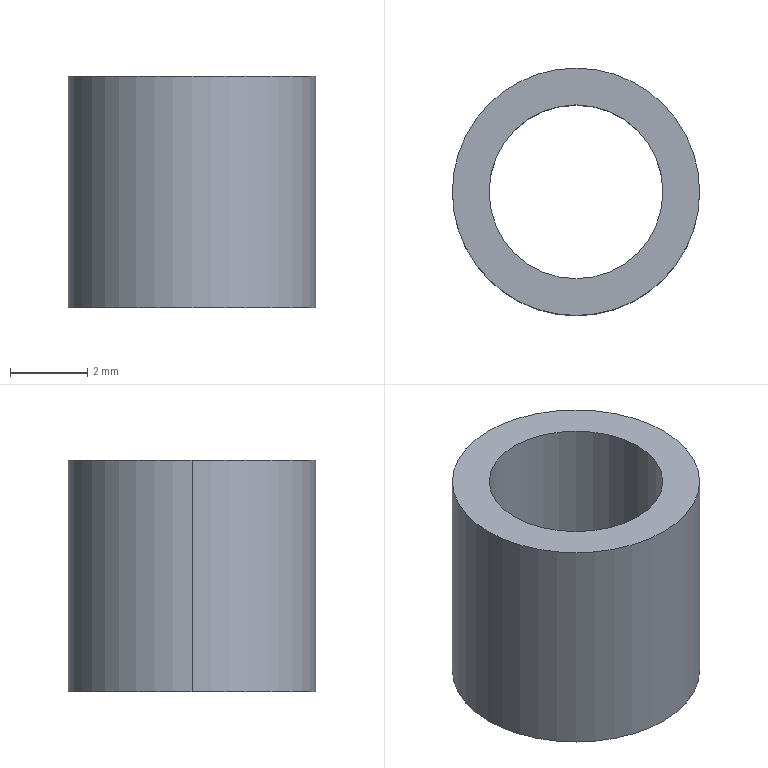Part | NX | features BREP 1 | 1 solid | 6 faces | box 6.4 x 6.4 x 6 mm | volume 97.594 mm3 | cylinder 4 | plane 2 | commonest cylinder face diameters 4.5 x2 6.4 x2
STEP:
#1=CARTESIAN_POINT('',(11.941,-8.741,33.83));
#2=VERTEX_POINT('',#1);
#3=CARTESIAN_POINT('',(5.541,-8.741,33.83));
#4=VERTEX_POINT('',#3);
#5=CARTESIAN_POINT('',(8.741,-8.741,33.83));
#6=DIRECTION('',(0.,0.,1.));
#7=DIRECTION('',(1.,0.,0.));
#8=AXIS2_PLACEMENT_3D('',#5,#6,#7);
#9=CIRCLE('',#8,3.2);
#10=EDGE_CURVE('',#2,#4,#9,.T.);
#11=ORIENTED_EDGE('',*,*,#10,.T.);
#12=CARTESIAN_POINT('',(8.741,-8.741,33.83));
#13=DIRECTION('',(0.,0.,1.));
#14=DIRECTION('',(-1.,0.,0.));
#15=AXIS2_PLACEMENT_3D('',#12,#13,#14);
#16=CIRCLE('',#15,3.2);
#17=EDGE_CURVE('',#4,#2,#16,.T.);
#18=ORIENTED_EDGE('',*,*,#17,.T.);
#19=EDGE_LOOP('',(#11,#18));
#20=FACE_BOUND('',#19,.T.);
#21=CARTESIAN_POINT('',(10.991,-8.741,33.83));
#22=VERTEX_POINT('',#21);
#23=CARTESIAN_POINT('',(6.491,-8.741,33.83));
#24=VERTEX_POINT('',#23);
#25=CARTESIAN_POINT('',(8.741,-8.741,33.83));
#26=DIRECTION('',(0.,0.,-1.));
#27=DIRECTION('',(1.,0.,0.));
#28=AXIS2_PLACEMENT_3D('',#25,#26,#27);
#29=CIRCLE('',#28,2.25);
#30=EDGE_CURVE('',#22,#24,#29,.T.);
#31=ORIENTED_EDGE('',*,*,#30,.T.);
#32=CARTESIAN_POINT('',(8.741,-8.741,33.83));
#33=DIRECTION('',(0.,0.,-1.));
#34=DIRECTION('',(-1.,0.,0.));
#35=AXIS2_PLACEMENT_3D('',#32,#33,#34);
#36=CIRCLE('',#35,2.25);
#37=EDGE_CURVE('',#24,#22,#36,.T.);
#38=ORIENTED_EDGE('',*,*,#37,.T.);
#39=EDGE_LOOP('',(#31,#38));
#40=FACE_BOUND('',#39,.T.);
#41=CARTESIAN_POINT('',(0.,0.,33.83));
#42=DIRECTION('',(0.,0.,1.));
#43=DIRECTION('',(1.,0.,0.));
#44=AXIS2_PLACEMENT_3D('',#41,#42,#43);
#45=PLANE('',#44);
#46=ADVANCED_FACE('',(#20,#40),#45,.T.);
#47=CARTESIAN_POINT('',(11.941,-8.741,27.83));
#48=VERTEX_POINT('',#47);
#49=CARTESIAN_POINT('',(5.541,-8.741,27.83));
#50=VERTEX_POINT('',#49);
#51=CARTESIAN_POINT('',(8.741,-8.741,27.83));
#52=DIRECTION('',(0.,0.,-1.));
#53=DIRECTION('',(1.,0.,0.));
#54=AXIS2_PLACEMENT_3D('',#51,#52,#53);
#55=CIRCLE('',#54,3.2);
#56=EDGE_CURVE('',#48,#50,#55,.T.);
#57=ORIENTED_EDGE('',*,*,#56,.F.);
#58=CARTESIAN_POINT('',(11.941,-8.741,33.83));
#59=DIRECTION('',(0.,0.,-1.));
#60=VECTOR('',#59,1000.);
#61=LINE('',#58,#60);
#62=EDGE_CURVE('',#2,#48,#61,.T.);
#63=ORIENTED_EDGE('',*,*,#62,.F.);
#64=ORIENTED_EDGE('',*,*,#17,.F.);
#65=CARTESIAN_POINT('',(5.541,-8.741,33.83));
#66=DIRECTION('',(0.,0.,-1.));
#67=VECTOR('',#66,1000.);
#68=LINE('',#65,#67);
#69=EDGE_CURVE('',#4,#50,#68,.T.);
#70=ORIENTED_EDGE('',*,*,#69,.T.);
#71=EDGE_LOOP('',(#57,#63,#64,#70));
#72=FACE_BOUND('',#71,.T.);
#73=CARTESIAN_POINT('',(8.741,-8.741,33.83));
#74=DIRECTION('',(0.,0.,1.));
#75=DIRECTION('',(1.,0.,0.));
#76=AXIS2_PLACEMENT_3D('',#73,#74,#75);
#77=CYLINDRICAL_SURFACE('',#76,3.2);
#78=ADVANCED_FACE('',(#72),#77,.T.);
#79=CARTESIAN_POINT('',(8.741,-8.741,27.83));
#80=DIRECTION('',(0.,0.,-1.));
#81=DIRECTION('',(-1.,0.,0.));
#82=AXIS2_PLACEMENT_3D('',#79,#80,#81);
#83=CIRCLE('',#82,3.2);
#84=EDGE_CURVE('',#50,#48,#83,.T.);
#85=ORIENTED_EDGE('',*,*,#84,.F.);
#86=ORIENTED_EDGE('',*,*,#69,.F.);
#87=ORIENTED_EDGE('',*,*,#10,.F.);
#88=ORIENTED_EDGE('',*,*,#62,.T.);
#89=EDGE_LOOP('',(#85,#86,#87,#88));
#90=FACE_BOUND('',#89,.T.);
#91=CARTESIAN_POINT('',(8.741,-8.741,33.83));
#92=DIRECTION('',(0.,0.,1.));
#93=DIRECTION('',(1.,0.,0.));
#94=AXIS2_PLACEMENT_3D('',#91,#92,#93);
#95=CYLINDRICAL_SURFACE('',#94,3.2);
#96=ADVANCED_FACE('',(#90),#95,.T.);
#97=ORIENTED_EDGE('',*,*,#84,.T.);
#98=ORIENTED_EDGE('',*,*,#56,.T.);
#99=EDGE_LOOP('',(#97,#98));
#100=FACE_BOUND('',#99,.T.);
#101=CARTESIAN_POINT('',(6.491,-8.741,27.83));
#102=VERTEX_POINT('',#101);
#103=CARTESIAN_POINT('',(10.991,-8.741,27.83));
#104=VERTEX_POINT('',#103);
#105=CARTESIAN_POINT('',(8.741,-8.741,27.83));
#106=DIRECTION('',(0.,0.,1.));
#107=DIRECTION('',(-1.,0.,0.));
#108=AXIS2_PLACEMENT_3D('',#105,#106,#107);
#109=CIRCLE('',#108,2.25);
#110=EDGE_CURVE('',#102,#104,#109,.T.);
#111=ORIENTED_EDGE('',*,*,#110,.T.);
#112=CARTESIAN_POINT('',(8.741,-8.741,27.83));
#113=DIRECTION('',(0.,0.,1.));
#114=DIRECTION('',(1.,0.,0.));
#115=AXIS2_PLACEMENT_3D('',#112,#113,#114);
#116=CIRCLE('',#115,2.25);
#117=EDGE_CURVE('',#104,#102,#116,.T.);
#118=ORIENTED_EDGE('',*,*,#117,.T.);
#119=EDGE_LOOP('',(#111,#118));
#120=FACE_BOUND('',#119,.T.);
#121=CARTESIAN_POINT('',(0.,0.,27.83));
#122=DIRECTION('',(0.,0.,1.));
#123=DIRECTION('',(1.,0.,0.));
#124=AXIS2_PLACEMENT_3D('',#121,#122,#123);
#125=PLANE('',#124);
#126=ADVANCED_FACE('',(#100,#120),#125,.F.);
#127=ORIENTED_EDGE('',*,*,#117,.F.);
#128=CARTESIAN_POINT('',(10.991,-8.741,33.83));
#129=DIRECTION('',(0.,0.,-1.));
#130=VECTOR('',#129,1000.);
#131=LINE('',#128,#130);
#132=EDGE_CURVE('',#22,#104,#131,.T.);
#133=ORIENTED_EDGE('',*,*,#132,.F.);
#134=ORIENTED_EDGE('',*,*,#37,.F.);
#135=CARTESIAN_POINT('',(6.491,-8.741,33.83));
#136=DIRECTION('',(0.,0.,-1.));
#137=VECTOR('',#136,1000.);
#138=LINE('',#135,#137);
#139=EDGE_CURVE('',#24,#102,#138,.T.);
#140=ORIENTED_EDGE('',*,*,#139,.T.);
#141=EDGE_LOOP('',(#127,#133,#134,#140));
#142=FACE_BOUND('',#141,.T.);
#143=CARTESIAN_POINT('',(8.741,-8.741,33.83));
#144=DIRECTION('',(0.,0.,1.));
#145=DIRECTION('',(1.,0.,0.));
#146=AXIS2_PLACEMENT_3D('',#143,#144,#145);
#147=CYLINDRICAL_SURFACE('',#146,2.25);
#148=ADVANCED_FACE('',(#142),#147,.F.);
#149=ORIENTED_EDGE('',*,*,#110,.F.);
#150=ORIENTED_EDGE('',*,*,#139,.F.);
#151=ORIENTED_EDGE('',*,*,#30,.F.);
#152=ORIENTED_EDGE('',*,*,#132,.T.);
#153=EDGE_LOOP('',(#149,#150,#151,#152));
#154=FACE_BOUND('',#153,.T.);
#155=CARTESIAN_POINT('',(8.741,-8.741,33.83));
#156=DIRECTION('',(0.,0.,1.));
#157=DIRECTION('',(1.,0.,0.));
#158=AXIS2_PLACEMENT_3D('',#155,#156,#157);
#159=CYLINDRICAL_SURFACE('',#158,2.25);
#160=ADVANCED_FACE('',(#154),#159,.F.);
#161=CLOSED_SHELL('',(#46,#78,#96,#126,#148,#160));
#162=MANIFOLD_SOLID_BREP('',#161);
#163=(LENGTH_UNIT()NAMED_UNIT(*)SI_UNIT(.MILLI.,.METRE.));
#164=UNCERTAINTY_MEASURE_WITH_UNIT(LENGTH_MEASURE(0.00001),#163,'','');
#165=(NAMED_UNIT(*)PLANE_ANGLE_UNIT()SI_UNIT($,.RADIAN.));
#166=(NAMED_UNIT(*)SI_UNIT($,.STERADIAN.)SOLID_ANGLE_UNIT());
#167=(GEOMETRIC_REPRESENTATION_CONTEXT(3)GLOBAL_UNCERTAINTY_ASSIGNED_CONTEXT((#164))GLOBAL_UNIT_ASSIGNED_CONTEXT((#163,#165,#166))REPRESENTATION_CONTEXT('',''));
#168=ADVANCED_BREP_SHAPE_REPRESENTATION('',(#162),#167);